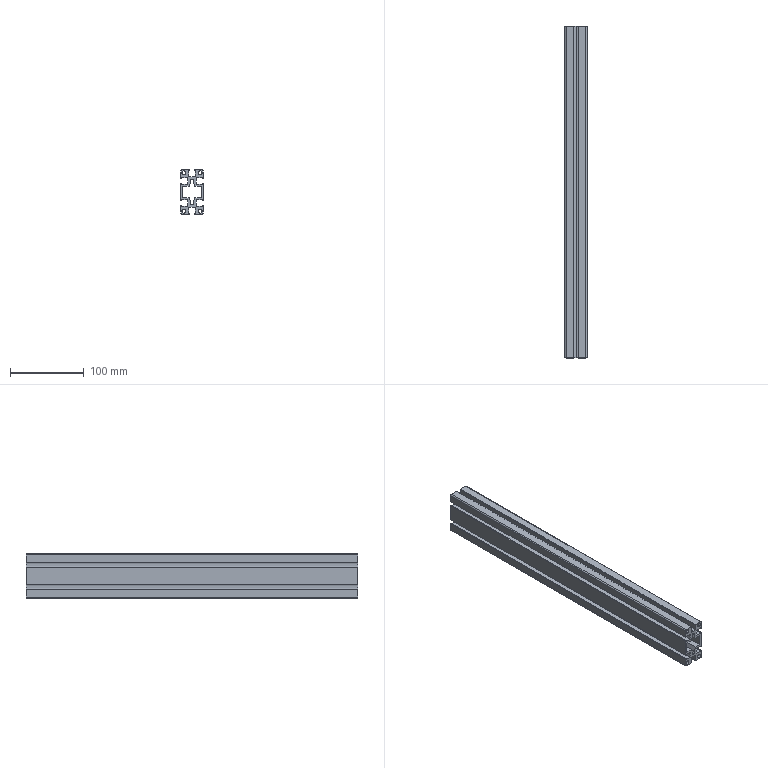Part | SolidWorks | features WeldMemberFeat 1, WeldmentFeature 1 | 1 solid | 80 faces | box 30 x 450 x 60 mm | volume 348814 mm3 | plane 58 | cylinder 22 | commonest cylinder face diameters 5.3 x8 24 x7 3 x4 5 x3